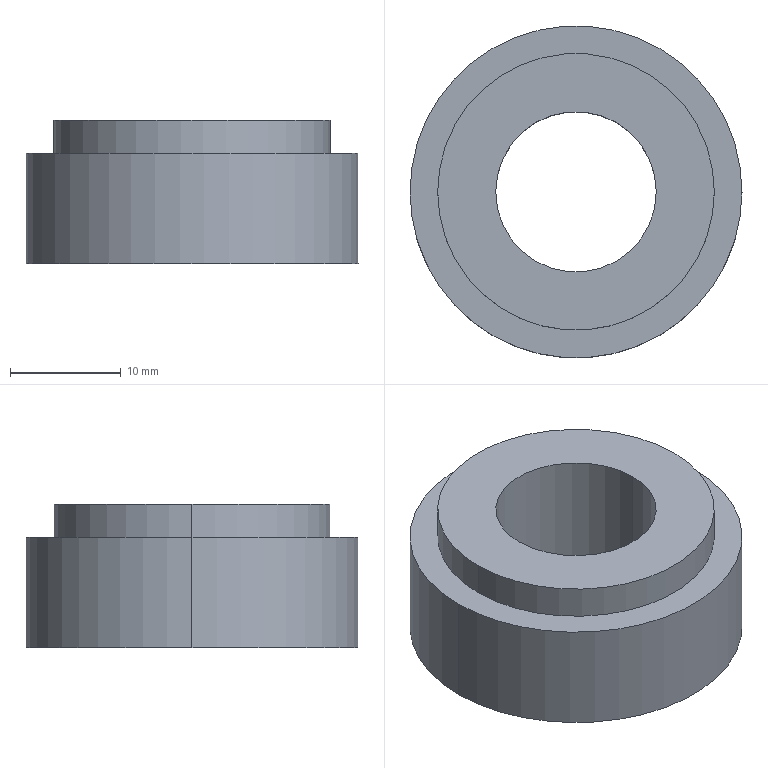Part | SolidWorks | features ICE 2, Extrusion 1, HoleWzd 1 | 1 solid | 9 faces | box 30 x 30 x 13 mm | volume 6395 mm3 | cylinder 6 | plane 3 | commonest cylinder face diameters 14.5 x2 25 x2 30 x2
STEP:
#1=CARTESIAN_POINT('',(-7.25,0.,13.));
#2=VERTEX_POINT('',#1);
#3=CARTESIAN_POINT('',(7.25,0.,13.));
#4=VERTEX_POINT('',#3);
#5=CARTESIAN_POINT('',(0.,0.,13.));
#6=DIRECTION('',(0.,0.,1.));
#7=DIRECTION('',(1.,0.,0.));
#8=AXIS2_PLACEMENT_3D('',#5,#6,#7);
#9=CIRCLE('',#8,7.25);
#10=EDGE_CURVE('',#2,#4,#9,.T.);
#11=ORIENTED_EDGE('',*,*,#10,.T.);
#12=CARTESIAN_POINT('',(7.25,0.,0.));
#13=VERTEX_POINT('',#12);
#14=CARTESIAN_POINT('',(7.25,0.,0.));
#15=DIRECTION('',(0.,0.,-1.));
#16=VECTOR('',#15,1000.);
#17=LINE('',#14,#16);
#18=EDGE_CURVE('',#4,#13,#17,.T.);
#19=ORIENTED_EDGE('',*,*,#18,.T.);
#20=CARTESIAN_POINT('',(-7.25,0.,0.));
#21=VERTEX_POINT('',#20);
#22=CARTESIAN_POINT('',(0.,0.,0.));
#23=DIRECTION('',(0.,0.,-1.));
#24=DIRECTION('',(-1.,0.,0.));
#25=AXIS2_PLACEMENT_3D('',#22,#23,#24);
#26=CIRCLE('',#25,7.25);
#27=EDGE_CURVE('',#13,#21,#26,.T.);
#28=ORIENTED_EDGE('',*,*,#27,.T.);
#29=CARTESIAN_POINT('',(-7.25,0.,0.));
#30=DIRECTION('',(0.,0.,-1.));
#31=VECTOR('',#30,1000.);
#32=LINE('',#29,#31);
#33=EDGE_CURVE('',#2,#21,#32,.T.);
#34=ORIENTED_EDGE('',*,*,#33,.F.);
#35=EDGE_LOOP('',(#11,#19,#28,#34));
#36=FACE_OUTER_BOUND('',#35,.T.);
#37=CARTESIAN_POINT('',(0.,0.,0.));
#38=DIRECTION('',(0.,0.,-1.));
#39=DIRECTION('',(-1.,0.,0.));
#40=AXIS2_PLACEMENT_3D('',#37,#38,#39);
#41=CYLINDRICAL_SURFACE('',#40,7.25);
#42=ADVANCED_FACE('',(#36),#41,.F.);
#43=CARTESIAN_POINT('',(12.5,0.,13.));
#44=VERTEX_POINT('',#43);
#45=CARTESIAN_POINT('',(-12.5,0.,13.));
#46=VERTEX_POINT('',#45);
#47=CARTESIAN_POINT('',(0.,0.,13.));
#48=DIRECTION('',(0.,0.,1.));
#49=DIRECTION('',(1.,0.,0.));
#50=AXIS2_PLACEMENT_3D('',#47,#48,#49);
#51=CIRCLE('',#50,12.5);
#52=EDGE_CURVE('',#44,#46,#51,.T.);
#53=ORIENTED_EDGE('',*,*,#52,.F.);
#54=CARTESIAN_POINT('',(12.5,0.,10.));
#55=VERTEX_POINT('',#54);
#56=CARTESIAN_POINT('',(12.5,0.,13.));
#57=DIRECTION('',(0.,0.,-1.));
#58=VECTOR('',#57,1000.);
#59=LINE('',#56,#58);
#60=EDGE_CURVE('',#44,#55,#59,.T.);
#61=ORIENTED_EDGE('',*,*,#60,.T.);
#62=CARTESIAN_POINT('',(-12.5,0.,10.));
#63=VERTEX_POINT('',#62);
#64=CARTESIAN_POINT('',(0.,0.,10.));
#65=DIRECTION('',(0.,0.,1.));
#66=DIRECTION('',(1.,0.,0.));
#67=AXIS2_PLACEMENT_3D('',#64,#65,#66);
#68=CIRCLE('',#67,12.5);
#69=EDGE_CURVE('',#55,#63,#68,.T.);
#70=ORIENTED_EDGE('',*,*,#69,.T.);
#71=CARTESIAN_POINT('',(-12.5,0.,13.));
#72=DIRECTION('',(0.,0.,-1.));
#73=VECTOR('',#72,1000.);
#74=LINE('',#71,#73);
#75=EDGE_CURVE('',#46,#63,#74,.T.);
#76=ORIENTED_EDGE('',*,*,#75,.F.);
#77=EDGE_LOOP('',(#53,#61,#70,#76));
#78=FACE_OUTER_BOUND('',#77,.T.);
#79=CARTESIAN_POINT('',(0.,0.,13.));
#80=DIRECTION('',(0.,0.,-1.));
#81=DIRECTION('',(-1.,0.,0.));
#82=AXIS2_PLACEMENT_3D('',#79,#80,#81);
#83=CYLINDRICAL_SURFACE('',#82,12.5);
#84=ADVANCED_FACE('',(#78),#83,.T.);
#85=CARTESIAN_POINT('',(15.,0.,10.));
#86=VERTEX_POINT('',#85);
#87=CARTESIAN_POINT('',(-15.,0.,10.));
#88=VERTEX_POINT('',#87);
#89=CARTESIAN_POINT('',(0.,0.,10.));
#90=DIRECTION('',(0.,0.,1.));
#91=DIRECTION('',(1.,0.,0.));
#92=AXIS2_PLACEMENT_3D('',#89,#90,#91);
#93=CIRCLE('',#92,15.);
#94=EDGE_CURVE('',#86,#88,#93,.T.);
#95=ORIENTED_EDGE('',*,*,#94,.F.);
#96=CARTESIAN_POINT('',(15.,0.,0.));
#97=VERTEX_POINT('',#96);
#98=CARTESIAN_POINT('',(15.,0.,10.));
#99=DIRECTION('',(0.,0.,-1.));
#100=VECTOR('',#99,1000.);
#101=LINE('',#98,#100);
#102=EDGE_CURVE('',#86,#97,#101,.T.);
#103=ORIENTED_EDGE('',*,*,#102,.T.);
#104=CARTESIAN_POINT('',(-15.,0.,0.));
#105=VERTEX_POINT('',#104);
#106=CARTESIAN_POINT('',(0.,0.,0.));
#107=DIRECTION('',(0.,0.,1.));
#108=DIRECTION('',(1.,0.,0.));
#109=AXIS2_PLACEMENT_3D('',#106,#107,#108);
#110=CIRCLE('',#109,15.);
#111=EDGE_CURVE('',#97,#105,#110,.T.);
#112=ORIENTED_EDGE('',*,*,#111,.T.);
#113=CARTESIAN_POINT('',(-15.,0.,10.));
#114=DIRECTION('',(0.,0.,-1.));
#115=VECTOR('',#114,1000.);
#116=LINE('',#113,#115);
#117=EDGE_CURVE('',#88,#105,#116,.T.);
#118=ORIENTED_EDGE('',*,*,#117,.F.);
#119=EDGE_LOOP('',(#95,#103,#112,#118));
#120=FACE_OUTER_BOUND('',#119,.T.);
#121=CARTESIAN_POINT('',(0.,0.,10.));
#122=DIRECTION('',(0.,0.,-1.));
#123=DIRECTION('',(-1.,0.,0.));
#124=AXIS2_PLACEMENT_3D('',#121,#122,#123);
#125=CYLINDRICAL_SURFACE('',#124,15.);
#126=ADVANCED_FACE('',(#120),#125,.T.);
#127=ORIENTED_EDGE('',*,*,#102,.F.);
#128=CARTESIAN_POINT('',(0.,0.,10.));
#129=DIRECTION('',(0.,0.,1.));
#130=DIRECTION('',(1.,0.,0.));
#131=AXIS2_PLACEMENT_3D('',#128,#129,#130);
#132=CIRCLE('',#131,15.);
#133=EDGE_CURVE('',#88,#86,#132,.T.);
#134=ORIENTED_EDGE('',*,*,#133,.F.);
#135=ORIENTED_EDGE('',*,*,#117,.T.);
#136=CARTESIAN_POINT('',(0.,0.,0.));
#137=DIRECTION('',(0.,0.,1.));
#138=DIRECTION('',(1.,0.,0.));
#139=AXIS2_PLACEMENT_3D('',#136,#137,#138);
#140=CIRCLE('',#139,15.);
#141=EDGE_CURVE('',#105,#97,#140,.T.);
#142=ORIENTED_EDGE('',*,*,#141,.T.);
#143=EDGE_LOOP('',(#127,#134,#135,#142));
#144=FACE_OUTER_BOUND('',#143,.T.);
#145=CARTESIAN_POINT('',(0.,0.,10.));
#146=DIRECTION('',(0.,0.,-1.));
#147=DIRECTION('',(-1.,0.,0.));
#148=AXIS2_PLACEMENT_3D('',#145,#146,#147);
#149=CYLINDRICAL_SURFACE('',#148,15.);
#150=ADVANCED_FACE('',(#144),#149,.T.);
#151=CARTESIAN_POINT('',(0.,0.,10.));
#152=DIRECTION('',(0.,0.,1.));
#153=DIRECTION('',(1.,0.,0.));
#154=AXIS2_PLACEMENT_3D('',#151,#152,#153);
#155=CIRCLE('',#154,12.5);
#156=EDGE_CURVE('',#63,#55,#155,.T.);
#157=ORIENTED_EDGE('',*,*,#156,.F.);
#158=ORIENTED_EDGE('',*,*,#69,.F.);
#159=EDGE_LOOP('',(#157,#158));
#160=FACE_BOUND('',#159,.T.);
#161=ORIENTED_EDGE('',*,*,#133,.T.);
#162=ORIENTED_EDGE('',*,*,#94,.T.);
#163=EDGE_LOOP('',(#161,#162));
#164=FACE_OUTER_BOUND('',#163,.T.);
#165=CARTESIAN_POINT('',(0.,0.,10.));
#166=DIRECTION('',(0.,0.,1.));
#167=DIRECTION('',(1.,0.,0.));
#168=AXIS2_PLACEMENT_3D('',#165,#166,#167);
#169=PLANE('',#168);
#170=ADVANCED_FACE('',(#160,#164),#169,.T.);
#171=CARTESIAN_POINT('',(0.,0.,0.));
#172=DIRECTION('',(0.,0.,-1.));
#173=DIRECTION('',(-1.,0.,0.));
#174=AXIS2_PLACEMENT_3D('',#171,#172,#173);
#175=CIRCLE('',#174,7.25);
#176=EDGE_CURVE('',#21,#13,#175,.T.);
#177=ORIENTED_EDGE('',*,*,#176,.F.);
#178=ORIENTED_EDGE('',*,*,#27,.F.);
#179=EDGE_LOOP('',(#177,#178));
#180=FACE_BOUND('',#179,.T.);
#181=ORIENTED_EDGE('',*,*,#141,.F.);
#182=ORIENTED_EDGE('',*,*,#111,.F.);
#183=EDGE_LOOP('',(#181,#182));
#184=FACE_OUTER_BOUND('',#183,.T.);
#185=CARTESIAN_POINT('',(0.,0.,0.));
#186=DIRECTION('',(0.,0.,1.));
#187=DIRECTION('',(1.,0.,0.));
#188=AXIS2_PLACEMENT_3D('',#185,#186,#187);
#189=PLANE('',#188);
#190=ADVANCED_FACE('',(#180,#184),#189,.F.);
#191=ORIENTED_EDGE('',*,*,#60,.F.);
#192=CARTESIAN_POINT('',(0.,0.,13.));
#193=DIRECTION('',(0.,0.,1.));
#194=DIRECTION('',(1.,0.,0.));
#195=AXIS2_PLACEMENT_3D('',#192,#193,#194);
#196=CIRCLE('',#195,12.5);
#197=EDGE_CURVE('',#46,#44,#196,.T.);
#198=ORIENTED_EDGE('',*,*,#197,.F.);
#199=ORIENTED_EDGE('',*,*,#75,.T.);
#200=ORIENTED_EDGE('',*,*,#156,.T.);
#201=EDGE_LOOP('',(#191,#198,#199,#200));
#202=FACE_OUTER_BOUND('',#201,.T.);
#203=CARTESIAN_POINT('',(0.,0.,13.));
#204=DIRECTION('',(0.,0.,-1.));
#205=DIRECTION('',(-1.,0.,0.));
#206=AXIS2_PLACEMENT_3D('',#203,#204,#205);
#207=CYLINDRICAL_SURFACE('',#206,12.5);
#208=ADVANCED_FACE('',(#202),#207,.T.);
#209=ORIENTED_EDGE('',*,*,#10,.F.);
#210=CARTESIAN_POINT('',(0.,0.,13.));
#211=DIRECTION('',(0.,0.,1.));
#212=DIRECTION('',(1.,0.,0.));
#213=AXIS2_PLACEMENT_3D('',#210,#211,#212);
#214=CIRCLE('',#213,7.25);
#215=EDGE_CURVE('',#4,#2,#214,.T.);
#216=ORIENTED_EDGE('',*,*,#215,.F.);
#217=EDGE_LOOP('',(#209,#216));
#218=FACE_BOUND('',#217,.T.);
#219=ORIENTED_EDGE('',*,*,#197,.T.);
#220=ORIENTED_EDGE('',*,*,#52,.T.);
#221=EDGE_LOOP('',(#219,#220));
#222=FACE_OUTER_BOUND('',#221,.T.);
#223=CARTESIAN_POINT('',(0.,0.,13.));
#224=DIRECTION('',(0.,0.,1.));
#225=DIRECTION('',(1.,0.,0.));
#226=AXIS2_PLACEMENT_3D('',#223,#224,#225);
#227=PLANE('',#226);
#228=ADVANCED_FACE('',(#218,#222),#227,.T.);
#229=ORIENTED_EDGE('',*,*,#18,.F.);
#230=ORIENTED_EDGE('',*,*,#215,.T.);
#231=ORIENTED_EDGE('',*,*,#33,.T.);
#232=ORIENTED_EDGE('',*,*,#176,.T.);
#233=EDGE_LOOP('',(#229,#230,#231,#232));
#234=FACE_OUTER_BOUND('',#233,.T.);
#235=CARTESIAN_POINT('',(0.,0.,0.));
#236=DIRECTION('',(0.,0.,-1.));
#237=DIRECTION('',(-1.,0.,0.));
#238=AXIS2_PLACEMENT_3D('',#235,#236,#237);
#239=CYLINDRICAL_SURFACE('',#238,7.25);
#240=ADVANCED_FACE('',(#234),#239,.F.);
#241=CLOSED_SHELL('',(#42,#84,#126,#150,#170,#190,#208,#228,#240));
#242=MANIFOLD_SOLID_BREP('',#241);
#243=CARTESIAN_POINT('',(0.,0.,0.));
#244=DIRECTION('',(0.,0.,1.));
#245=DIRECTION('',(1.,0.,0.));
#246=AXIS2_PLACEMENT_3D('',#243,#244,#245);
#247=(LENGTH_UNIT()NAMED_UNIT(*)SI_UNIT(.MILLI.,.METRE.));
#248=UNCERTAINTY_MEASURE_WITH_UNIT(LENGTH_MEASURE(0.00001),#247,'','');
#249=(NAMED_UNIT(*)PLANE_ANGLE_UNIT()SI_UNIT($,.RADIAN.));
#250=(NAMED_UNIT(*)SI_UNIT($,.STERADIAN.)SOLID_ANGLE_UNIT());
#251=(GEOMETRIC_REPRESENTATION_CONTEXT(3)GLOBAL_UNCERTAINTY_ASSIGNED_CONTEXT((#248))GLOBAL_UNIT_ASSIGNED_CONTEXT((#247,#249,#250))REPRESENTATION_CONTEXT('',''));
#252=ADVANCED_BREP_SHAPE_REPRESENTATION('',(#242,#246),#251);